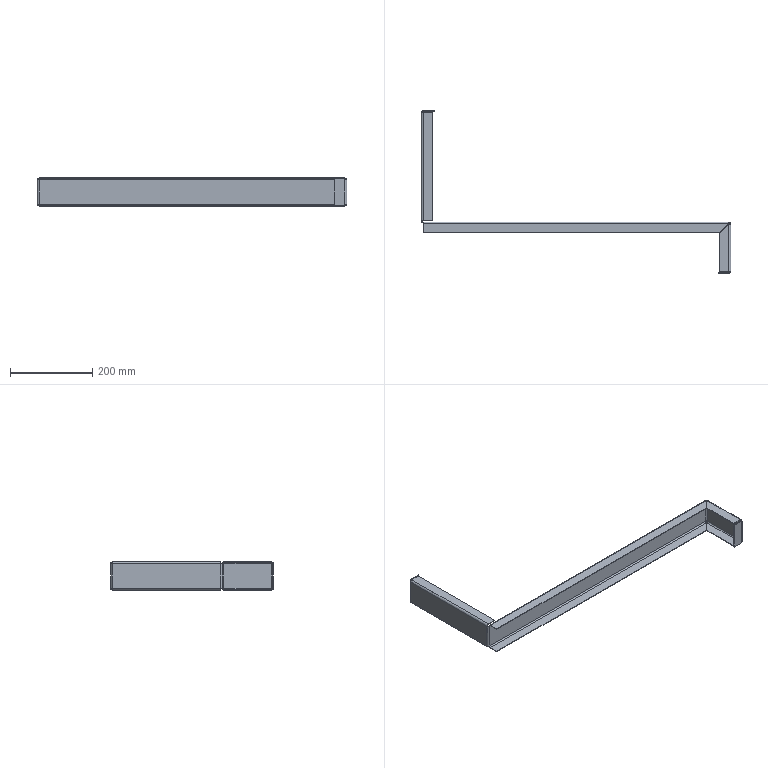Part | SolidWorks | features BaseBody 1 | 1 solid | 90 faces | box 751.5 x 394 x 68 mm | volume 198478 mm3 | plane 66 | cylinder 20 | spline 4 | commonest cylinder face diameters 6 x10 9 x10